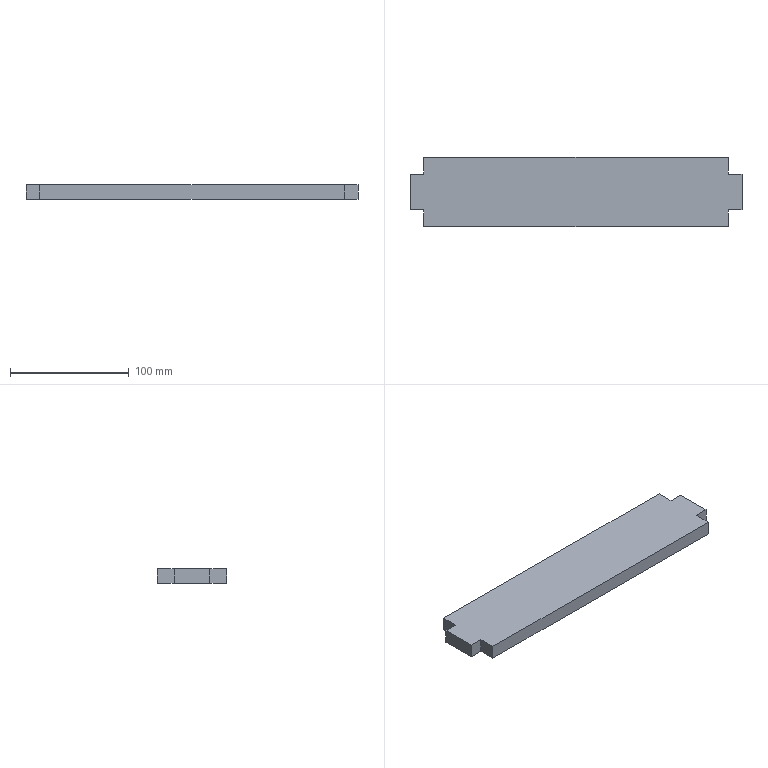Part | SolidWorks | features FlatPattern 1, SMBaseFlange 1, SheetMetal 1 | 1 solid | 14 faces | box 279 x 58.5 x 12 mm | volume 187992 mm3 | plane 14
STEP:
#1=CARTESIAN_POINT('',(-165.445,-124.118,0.));
#2=VERTEX_POINT('',#1);
#3=CARTESIAN_POINT('',(-165.445,-138.368,0.));
#4=VERTEX_POINT('',#3);
#5=CARTESIAN_POINT('',(-165.445,-124.118,0.));
#6=DIRECTION('',(0.,-1.,0.));
#7=VECTOR('',#6,1000.);
#8=LINE('',#5,#7);
#9=EDGE_CURVE('',#2,#4,#8,.T.);
#10=ORIENTED_EDGE('',*,*,#9,.T.);
#11=CARTESIAN_POINT('',(-165.445,-138.368,12.));
#12=VERTEX_POINT('',#11);
#13=CARTESIAN_POINT('',(-165.445,-138.368,12.));
#14=DIRECTION('',(0.,0.,-1.));
#15=VECTOR('',#14,1000.);
#16=LINE('',#13,#15);
#17=EDGE_CURVE('',#12,#4,#16,.T.);
#18=ORIENTED_EDGE('',*,*,#17,.F.);
#19=CARTESIAN_POINT('',(-165.445,-124.118,12.));
#20=VERTEX_POINT('',#19);
#21=CARTESIAN_POINT('',(-165.445,-124.118,12.));
#22=DIRECTION('',(0.,-1.,0.));
#23=VECTOR('',#22,1000.);
#24=LINE('',#21,#23);
#25=EDGE_CURVE('',#20,#12,#24,.T.);
#26=ORIENTED_EDGE('',*,*,#25,.F.);
#27=CARTESIAN_POINT('',(-165.445,-124.118,12.));
#28=DIRECTION('',(0.,0.,-1.));
#29=VECTOR('',#28,1000.);
#30=LINE('',#27,#29);
#31=EDGE_CURVE('',#20,#2,#30,.T.);
#32=ORIENTED_EDGE('',*,*,#31,.T.);
#33=EDGE_LOOP('',(#10,#18,#26,#32));
#34=FACE_OUTER_BOUND('',#33,.T.);
#35=CARTESIAN_POINT('',(-165.445,-124.118,12.));
#36=DIRECTION('',(1.,0.,0.));
#37=DIRECTION('',(0.,0.,-1.));
#38=AXIS2_PLACEMENT_3D('',#35,#36,#37);
#39=PLANE('',#38);
#40=ADVANCED_FACE('',(#34),#39,.F.);
#41=CARTESIAN_POINT('',(-176.945,-138.368,0.));
#42=VERTEX_POINT('',#41);
#43=CARTESIAN_POINT('',(-165.445,-138.368,0.));
#44=DIRECTION('',(-1.,0.,0.));
#45=VECTOR('',#44,1000.);
#46=LINE('',#43,#45);
#47=EDGE_CURVE('',#4,#42,#46,.T.);
#48=ORIENTED_EDGE('',*,*,#47,.T.);
#49=CARTESIAN_POINT('',(-176.945,-138.368,12.));
#50=VERTEX_POINT('',#49);
#51=CARTESIAN_POINT('',(-176.945,-138.368,12.));
#52=DIRECTION('',(0.,0.,-1.));
#53=VECTOR('',#52,1000.);
#54=LINE('',#51,#53);
#55=EDGE_CURVE('',#50,#42,#54,.T.);
#56=ORIENTED_EDGE('',*,*,#55,.F.);
#57=CARTESIAN_POINT('',(-165.445,-138.368,12.));
#58=DIRECTION('',(-1.,0.,0.));
#59=VECTOR('',#58,1000.);
#60=LINE('',#57,#59);
#61=EDGE_CURVE('',#12,#50,#60,.T.);
#62=ORIENTED_EDGE('',*,*,#61,.F.);
#63=ORIENTED_EDGE('',*,*,#17,.T.);
#64=EDGE_LOOP('',(#48,#56,#62,#63));
#65=FACE_OUTER_BOUND('',#64,.T.);
#66=CARTESIAN_POINT('',(-165.445,-138.368,12.));
#67=DIRECTION('',(0.,-1.,0.));
#68=DIRECTION('',(0.,0.,-1.));
#69=AXIS2_PLACEMENT_3D('',#66,#67,#68);
#70=PLANE('',#69);
#71=ADVANCED_FACE('',(#65),#70,.F.);
#72=CARTESIAN_POINT('',(-176.945,-168.368,0.));
#73=VERTEX_POINT('',#72);
#74=CARTESIAN_POINT('',(-176.945,-138.368,0.));
#75=DIRECTION('',(0.,-1.,0.));
#76=VECTOR('',#75,1000.);
#77=LINE('',#74,#76);
#78=EDGE_CURVE('',#42,#73,#77,.T.);
#79=ORIENTED_EDGE('',*,*,#78,.T.);
#80=CARTESIAN_POINT('',(-176.945,-168.368,12.));
#81=VERTEX_POINT('',#80);
#82=CARTESIAN_POINT('',(-176.945,-168.368,12.));
#83=DIRECTION('',(0.,0.,-1.));
#84=VECTOR('',#83,1000.);
#85=LINE('',#82,#84);
#86=EDGE_CURVE('',#81,#73,#85,.T.);
#87=ORIENTED_EDGE('',*,*,#86,.F.);
#88=CARTESIAN_POINT('',(-176.945,-138.368,12.));
#89=DIRECTION('',(0.,-1.,0.));
#90=VECTOR('',#89,1000.);
#91=LINE('',#88,#90);
#92=EDGE_CURVE('',#50,#81,#91,.T.);
#93=ORIENTED_EDGE('',*,*,#92,.F.);
#94=ORIENTED_EDGE('',*,*,#55,.T.);
#95=EDGE_LOOP('',(#79,#87,#93,#94));
#96=FACE_OUTER_BOUND('',#95,.T.);
#97=CARTESIAN_POINT('',(-176.945,-138.368,12.));
#98=DIRECTION('',(1.,0.,0.));
#99=DIRECTION('',(0.,0.,-1.));
#100=AXIS2_PLACEMENT_3D('',#97,#98,#99);
#101=PLANE('',#100);
#102=ADVANCED_FACE('',(#96),#101,.F.);
#103=CARTESIAN_POINT('',(-165.445,-168.368,0.));
#104=VERTEX_POINT('',#103);
#105=CARTESIAN_POINT('',(-176.945,-168.368,0.));
#106=DIRECTION('',(1.,0.,0.));
#107=VECTOR('',#106,1000.);
#108=LINE('',#105,#107);
#109=EDGE_CURVE('',#73,#104,#108,.T.);
#110=ORIENTED_EDGE('',*,*,#109,.T.);
#111=CARTESIAN_POINT('',(-165.445,-168.368,12.));
#112=VERTEX_POINT('',#111);
#113=CARTESIAN_POINT('',(-165.445,-168.368,12.));
#114=DIRECTION('',(0.,0.,-1.));
#115=VECTOR('',#114,1000.);
#116=LINE('',#113,#115);
#117=EDGE_CURVE('',#112,#104,#116,.T.);
#118=ORIENTED_EDGE('',*,*,#117,.F.);
#119=CARTESIAN_POINT('',(-176.945,-168.368,12.));
#120=DIRECTION('',(1.,0.,0.));
#121=VECTOR('',#120,1000.);
#122=LINE('',#119,#121);
#123=EDGE_CURVE('',#81,#112,#122,.T.);
#124=ORIENTED_EDGE('',*,*,#123,.F.);
#125=ORIENTED_EDGE('',*,*,#86,.T.);
#126=EDGE_LOOP('',(#110,#118,#124,#125));
#127=FACE_OUTER_BOUND('',#126,.T.);
#128=CARTESIAN_POINT('',(-176.945,-168.368,12.));
#129=DIRECTION('',(0.,1.,0.));
#130=DIRECTION('',(0.,0.,1.));
#131=AXIS2_PLACEMENT_3D('',#128,#129,#130);
#132=PLANE('',#131);
#133=ADVANCED_FACE('',(#127),#132,.F.);
#134=CARTESIAN_POINT('',(-165.445,-182.618,0.));
#135=VERTEX_POINT('',#134);
#136=CARTESIAN_POINT('',(-165.445,-168.368,0.));
#137=DIRECTION('',(0.,-1.,0.));
#138=VECTOR('',#137,1000.);
#139=LINE('',#136,#138);
#140=EDGE_CURVE('',#104,#135,#139,.T.);
#141=ORIENTED_EDGE('',*,*,#140,.T.);
#142=CARTESIAN_POINT('',(-165.445,-182.618,12.));
#143=VERTEX_POINT('',#142);
#144=CARTESIAN_POINT('',(-165.445,-182.618,12.));
#145=DIRECTION('',(0.,0.,-1.));
#146=VECTOR('',#145,1000.);
#147=LINE('',#144,#146);
#148=EDGE_CURVE('',#143,#135,#147,.T.);
#149=ORIENTED_EDGE('',*,*,#148,.F.);
#150=CARTESIAN_POINT('',(-165.445,-168.368,12.));
#151=DIRECTION('',(0.,-1.,0.));
#152=VECTOR('',#151,1000.);
#153=LINE('',#150,#152);
#154=EDGE_CURVE('',#112,#143,#153,.T.);
#155=ORIENTED_EDGE('',*,*,#154,.F.);
#156=ORIENTED_EDGE('',*,*,#117,.T.);
#157=EDGE_LOOP('',(#141,#149,#155,#156));
#158=FACE_OUTER_BOUND('',#157,.T.);
#159=CARTESIAN_POINT('',(-165.445,-168.368,12.));
#160=DIRECTION('',(1.,0.,0.));
#161=DIRECTION('',(0.,1.,0.));
#162=AXIS2_PLACEMENT_3D('',#159,#160,#161);
#163=PLANE('',#162);
#164=ADVANCED_FACE('',(#158),#163,.F.);
#165=CARTESIAN_POINT('',(90.555,-182.618,0.));
#166=VERTEX_POINT('',#165);
#167=CARTESIAN_POINT('',(-165.445,-182.618,0.));
#168=DIRECTION('',(1.,0.,0.));
#169=VECTOR('',#168,1000.);
#170=LINE('',#167,#169);
#171=EDGE_CURVE('',#135,#166,#170,.T.);
#172=ORIENTED_EDGE('',*,*,#171,.T.);
#173=CARTESIAN_POINT('',(90.555,-182.618,12.));
#174=VERTEX_POINT('',#173);
#175=CARTESIAN_POINT('',(90.555,-182.618,12.));
#176=DIRECTION('',(0.,0.,-1.));
#177=VECTOR('',#176,1000.);
#178=LINE('',#175,#177);
#179=EDGE_CURVE('',#174,#166,#178,.T.);
#180=ORIENTED_EDGE('',*,*,#179,.F.);
#181=CARTESIAN_POINT('',(-165.445,-182.618,12.));
#182=DIRECTION('',(1.,0.,0.));
#183=VECTOR('',#182,1000.);
#184=LINE('',#181,#183);
#185=EDGE_CURVE('',#143,#174,#184,.T.);
#186=ORIENTED_EDGE('',*,*,#185,.F.);
#187=ORIENTED_EDGE('',*,*,#148,.T.);
#188=EDGE_LOOP('',(#172,#180,#186,#187));
#189=FACE_OUTER_BOUND('',#188,.T.);
#190=CARTESIAN_POINT('',(-165.445,-182.618,12.));
#191=DIRECTION('',(0.,1.,0.));
#192=DIRECTION('',(0.,0.,1.));
#193=AXIS2_PLACEMENT_3D('',#190,#191,#192);
#194=PLANE('',#193);
#195=ADVANCED_FACE('',(#189),#194,.F.);
#196=CARTESIAN_POINT('',(90.555,-168.368,0.));
#197=VERTEX_POINT('',#196);
#198=CARTESIAN_POINT('',(90.555,-168.368,0.));
#199=DIRECTION('',(0.,1.,0.));
#200=VECTOR('',#199,1000.);
#201=LINE('',#198,#200);
#202=EDGE_CURVE('',#166,#197,#201,.T.);
#203=ORIENTED_EDGE('',*,*,#202,.T.);
#204=CARTESIAN_POINT('',(90.555,-168.368,12.));
#205=VERTEX_POINT('',#204);
#206=CARTESIAN_POINT('',(90.555,-168.368,12.));
#207=DIRECTION('',(0.,0.,-1.));
#208=VECTOR('',#207,1000.);
#209=LINE('',#206,#208);
#210=EDGE_CURVE('',#205,#197,#209,.T.);
#211=ORIENTED_EDGE('',*,*,#210,.F.);
#212=CARTESIAN_POINT('',(90.555,-168.368,12.));
#213=DIRECTION('',(0.,1.,0.));
#214=VECTOR('',#213,1000.);
#215=LINE('',#212,#214);
#216=EDGE_CURVE('',#174,#205,#215,.T.);
#217=ORIENTED_EDGE('',*,*,#216,.F.);
#218=ORIENTED_EDGE('',*,*,#179,.T.);
#219=EDGE_LOOP('',(#203,#211,#217,#218));
#220=FACE_OUTER_BOUND('',#219,.T.);
#221=CARTESIAN_POINT('',(90.555,-168.368,12.));
#222=DIRECTION('',(-1.,0.,0.));
#223=DIRECTION('',(0.,0.,1.));
#224=AXIS2_PLACEMENT_3D('',#221,#222,#223);
#225=PLANE('',#224);
#226=ADVANCED_FACE('',(#220),#225,.F.);
#227=CARTESIAN_POINT('',(102.055,-168.368,0.));
#228=VERTEX_POINT('',#227);
#229=CARTESIAN_POINT('',(102.055,-168.368,0.));
#230=DIRECTION('',(1.,0.,0.));
#231=VECTOR('',#230,1000.);
#232=LINE('',#229,#231);
#233=EDGE_CURVE('',#197,#228,#232,.T.);
#234=ORIENTED_EDGE('',*,*,#233,.T.);
#235=CARTESIAN_POINT('',(102.055,-168.368,12.));
#236=VERTEX_POINT('',#235);
#237=CARTESIAN_POINT('',(102.055,-168.368,12.));
#238=DIRECTION('',(0.,0.,-1.));
#239=VECTOR('',#238,1000.);
#240=LINE('',#237,#239);
#241=EDGE_CURVE('',#236,#228,#240,.T.);
#242=ORIENTED_EDGE('',*,*,#241,.F.);
#243=CARTESIAN_POINT('',(102.055,-168.368,12.));
#244=DIRECTION('',(1.,0.,0.));
#245=VECTOR('',#244,1000.);
#246=LINE('',#243,#245);
#247=EDGE_CURVE('',#205,#236,#246,.T.);
#248=ORIENTED_EDGE('',*,*,#247,.F.);
#249=ORIENTED_EDGE('',*,*,#210,.T.);
#250=EDGE_LOOP('',(#234,#242,#248,#249));
#251=FACE_OUTER_BOUND('',#250,.T.);
#252=CARTESIAN_POINT('',(102.055,-168.368,12.));
#253=DIRECTION('',(0.,1.,0.));
#254=DIRECTION('',(0.,0.,1.));
#255=AXIS2_PLACEMENT_3D('',#252,#253,#254);
#256=PLANE('',#255);
#257=ADVANCED_FACE('',(#251),#256,.F.);
#258=CARTESIAN_POINT('',(102.055,-138.368,0.));
#259=VERTEX_POINT('',#258);
#260=CARTESIAN_POINT('',(102.055,-138.368,0.));
#261=DIRECTION('',(0.,1.,0.));
#262=VECTOR('',#261,1000.);
#263=LINE('',#260,#262);
#264=EDGE_CURVE('',#228,#259,#263,.T.);
#265=ORIENTED_EDGE('',*,*,#264,.T.);
#266=CARTESIAN_POINT('',(102.055,-138.368,12.));
#267=VERTEX_POINT('',#266);
#268=CARTESIAN_POINT('',(102.055,-138.368,12.));
#269=DIRECTION('',(0.,0.,-1.));
#270=VECTOR('',#269,1000.);
#271=LINE('',#268,#270);
#272=EDGE_CURVE('',#267,#259,#271,.T.);
#273=ORIENTED_EDGE('',*,*,#272,.F.);
#274=CARTESIAN_POINT('',(102.055,-138.368,12.));
#275=DIRECTION('',(0.,1.,0.));
#276=VECTOR('',#275,1000.);
#277=LINE('',#274,#276);
#278=EDGE_CURVE('',#236,#267,#277,.T.);
#279=ORIENTED_EDGE('',*,*,#278,.F.);
#280=ORIENTED_EDGE('',*,*,#241,.T.);
#281=EDGE_LOOP('',(#265,#273,#279,#280));
#282=FACE_OUTER_BOUND('',#281,.T.);
#283=CARTESIAN_POINT('',(102.055,-138.368,12.));
#284=DIRECTION('',(-1.,0.,0.));
#285=DIRECTION('',(0.,0.,1.));
#286=AXIS2_PLACEMENT_3D('',#283,#284,#285);
#287=PLANE('',#286);
#288=ADVANCED_FACE('',(#282),#287,.F.);
#289=CARTESIAN_POINT('',(90.555,-138.368,0.));
#290=VERTEX_POINT('',#289);
#291=CARTESIAN_POINT('',(90.555,-138.368,0.));
#292=DIRECTION('',(-1.,0.,0.));
#293=VECTOR('',#292,1000.);
#294=LINE('',#291,#293);
#295=EDGE_CURVE('',#259,#290,#294,.T.);
#296=ORIENTED_EDGE('',*,*,#295,.T.);
#297=CARTESIAN_POINT('',(90.555,-138.368,12.));
#298=VERTEX_POINT('',#297);
#299=CARTESIAN_POINT('',(90.555,-138.368,12.));
#300=DIRECTION('',(0.,0.,-1.));
#301=VECTOR('',#300,1000.);
#302=LINE('',#299,#301);
#303=EDGE_CURVE('',#298,#290,#302,.T.);
#304=ORIENTED_EDGE('',*,*,#303,.F.);
#305=CARTESIAN_POINT('',(90.555,-138.368,12.));
#306=DIRECTION('',(-1.,0.,0.));
#307=VECTOR('',#306,1000.);
#308=LINE('',#305,#307);
#309=EDGE_CURVE('',#267,#298,#308,.T.);
#310=ORIENTED_EDGE('',*,*,#309,.F.);
#311=ORIENTED_EDGE('',*,*,#272,.T.);
#312=EDGE_LOOP('',(#296,#304,#310,#311));
#313=FACE_OUTER_BOUND('',#312,.T.);
#314=CARTESIAN_POINT('',(90.555,-138.368,12.));
#315=DIRECTION('',(0.,-1.,0.));
#316=DIRECTION('',(0.,0.,-1.));
#317=AXIS2_PLACEMENT_3D('',#314,#315,#316);
#318=PLANE('',#317);
#319=ADVANCED_FACE('',(#313),#318,.F.);
#320=CARTESIAN_POINT('',(90.555,-124.118,0.));
#321=VERTEX_POINT('',#320);
#322=CARTESIAN_POINT('',(90.555,-124.118,0.));
#323=DIRECTION('',(0.,1.,0.));
#324=VECTOR('',#323,1000.);
#325=LINE('',#322,#324);
#326=EDGE_CURVE('',#290,#321,#325,.T.);
#327=ORIENTED_EDGE('',*,*,#326,.T.);
#328=CARTESIAN_POINT('',(90.555,-124.118,12.));
#329=VERTEX_POINT('',#328);
#330=CARTESIAN_POINT('',(90.555,-124.118,12.));
#331=DIRECTION('',(0.,0.,-1.));
#332=VECTOR('',#331,1000.);
#333=LINE('',#330,#332);
#334=EDGE_CURVE('',#329,#321,#333,.T.);
#335=ORIENTED_EDGE('',*,*,#334,.F.);
#336=CARTESIAN_POINT('',(90.555,-124.118,12.));
#337=DIRECTION('',(0.,1.,0.));
#338=VECTOR('',#337,1000.);
#339=LINE('',#336,#338);
#340=EDGE_CURVE('',#298,#329,#339,.T.);
#341=ORIENTED_EDGE('',*,*,#340,.F.);
#342=ORIENTED_EDGE('',*,*,#303,.T.);
#343=EDGE_LOOP('',(#327,#335,#341,#342));
#344=FACE_OUTER_BOUND('',#343,.T.);
#345=CARTESIAN_POINT('',(90.555,-124.118,12.));
#346=DIRECTION('',(-1.,0.,0.));
#347=DIRECTION('',(0.,-1.,0.));
#348=AXIS2_PLACEMENT_3D('',#345,#346,#347);
#349=PLANE('',#348);
#350=ADVANCED_FACE('',(#344),#349,.F.);
#351=CARTESIAN_POINT('',(-165.445,-124.118,0.));
#352=DIRECTION('',(-1.,0.,0.));
#353=VECTOR('',#352,1000.);
#354=LINE('',#351,#353);
#355=EDGE_CURVE('',#321,#2,#354,.T.);
#356=ORIENTED_EDGE('',*,*,#355,.T.);
#357=ORIENTED_EDGE('',*,*,#31,.F.);
#358=CARTESIAN_POINT('',(-165.445,-124.118,12.));
#359=DIRECTION('',(-1.,0.,0.));
#360=VECTOR('',#359,1000.);
#361=LINE('',#358,#360);
#362=EDGE_CURVE('',#329,#20,#361,.T.);
#363=ORIENTED_EDGE('',*,*,#362,.F.);
#364=ORIENTED_EDGE('',*,*,#334,.T.);
#365=EDGE_LOOP('',(#356,#357,#363,#364));
#366=FACE_OUTER_BOUND('',#365,.T.);
#367=CARTESIAN_POINT('',(-165.445,-124.118,12.));
#368=DIRECTION('',(0.,-1.,0.));
#369=DIRECTION('',(0.,0.,-1.));
#370=AXIS2_PLACEMENT_3D('',#367,#368,#369);
#371=PLANE('',#370);
#372=ADVANCED_FACE('',(#366),#371,.F.);
#373=ORIENTED_EDGE('',*,*,#25,.T.);
#374=ORIENTED_EDGE('',*,*,#61,.T.);
#375=ORIENTED_EDGE('',*,*,#92,.T.);
#376=ORIENTED_EDGE('',*,*,#123,.T.);
#377=ORIENTED_EDGE('',*,*,#154,.T.);
#378=ORIENTED_EDGE('',*,*,#185,.T.);
#379=ORIENTED_EDGE('',*,*,#216,.T.);
#380=ORIENTED_EDGE('',*,*,#247,.T.);
#381=ORIENTED_EDGE('',*,*,#278,.T.);
#382=ORIENTED_EDGE('',*,*,#309,.T.);
#383=ORIENTED_EDGE('',*,*,#340,.T.);
#384=ORIENTED_EDGE('',*,*,#362,.T.);
#385=EDGE_LOOP('',(#373,#374,#375,#376,#377,#378,#379,#380,#381,#382,#383,#384));
#386=FACE_OUTER_BOUND('',#385,.T.);
#387=CARTESIAN_POINT('',(0.,0.,12.));
#388=DIRECTION('',(0.,0.,-1.));
#389=DIRECTION('',(-1.,0.,0.));
#390=AXIS2_PLACEMENT_3D('',#387,#388,#389);
#391=PLANE('',#390);
#392=ADVANCED_FACE('',(#386),#391,.F.);
#393=ORIENTED_EDGE('',*,*,#9,.F.);
#394=ORIENTED_EDGE('',*,*,#355,.F.);
#395=ORIENTED_EDGE('',*,*,#326,.F.);
#396=ORIENTED_EDGE('',*,*,#295,.F.);
#397=ORIENTED_EDGE('',*,*,#264,.F.);
#398=ORIENTED_EDGE('',*,*,#233,.F.);
#399=ORIENTED_EDGE('',*,*,#202,.F.);
#400=ORIENTED_EDGE('',*,*,#171,.F.);
#401=ORIENTED_EDGE('',*,*,#140,.F.);
#402=ORIENTED_EDGE('',*,*,#109,.F.);
#403=ORIENTED_EDGE('',*,*,#78,.F.);
#404=ORIENTED_EDGE('',*,*,#47,.F.);
#405=EDGE_LOOP('',(#393,#394,#395,#396,#397,#398,#399,#400,#401,#402,#403,#404));
#406=FACE_OUTER_BOUND('',#405,.T.);
#407=CARTESIAN_POINT('',(0.,0.,0.));
#408=DIRECTION('',(0.,0.,-1.));
#409=DIRECTION('',(-1.,0.,0.));
#410=AXIS2_PLACEMENT_3D('',#407,#408,#409);
#411=PLANE('',#410);
#412=ADVANCED_FACE('',(#406),#411,.T.);
#413=CLOSED_SHELL('',(#40,#71,#102,#133,#164,#195,#226,#257,#288,#319,#350,#372,#392,#412));
#414=MANIFOLD_SOLID_BREP('',#413);
#415=CARTESIAN_POINT('',(0.,0.,0.));
#416=DIRECTION('',(0.,0.,1.));
#417=DIRECTION('',(1.,0.,0.));
#418=AXIS2_PLACEMENT_3D('',#415,#416,#417);
#419=(LENGTH_UNIT()NAMED_UNIT(*)SI_UNIT(.MILLI.,.METRE.));
#420=UNCERTAINTY_MEASURE_WITH_UNIT(LENGTH_MEASURE(0.00001),#419,'','');
#421=(NAMED_UNIT(*)PLANE_ANGLE_UNIT()SI_UNIT($,.RADIAN.));
#422=(NAMED_UNIT(*)SI_UNIT($,.STERADIAN.)SOLID_ANGLE_UNIT());
#423=(GEOMETRIC_REPRESENTATION_CONTEXT(3)GLOBAL_UNCERTAINTY_ASSIGNED_CONTEXT((#420))GLOBAL_UNIT_ASSIGNED_CONTEXT((#419,#421,#422))REPRESENTATION_CONTEXT('',''));
#424=ADVANCED_BREP_SHAPE_REPRESENTATION('',(#414,#418),#423);